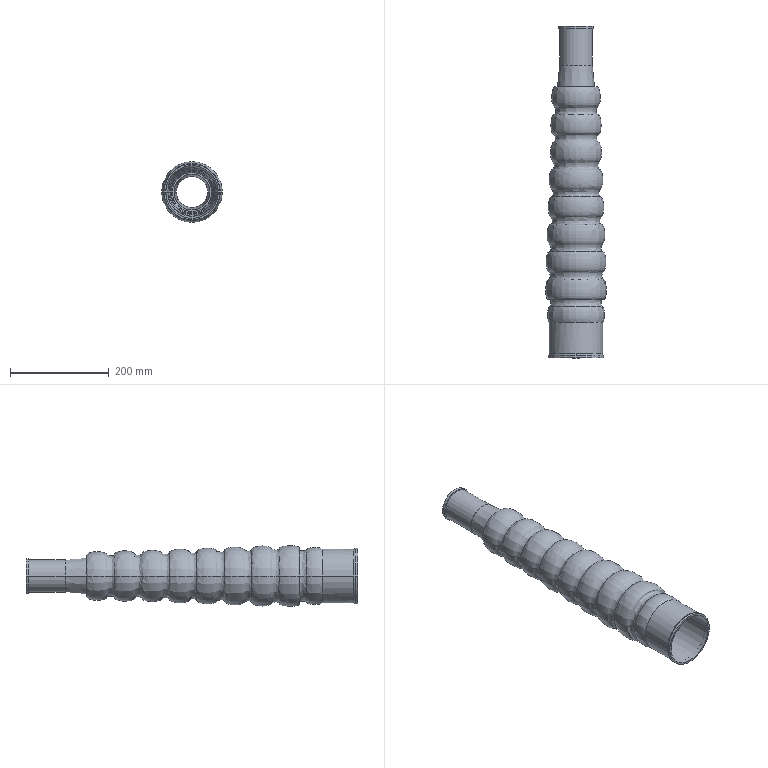Part | STEP file | Electric cylinder dust boot, cylinder B | 1 solid | 60 faces | box 122.855 x 671.584 x 122.855 mm | volume 479397 mm3 | spline 38 | cylinder 12 | plane 6 | cone 4 | commonest cylinder face diameters 63.286 x2 66.286 x2 70.625 x2 106.253 x2 109.253 x2 113.178 x2